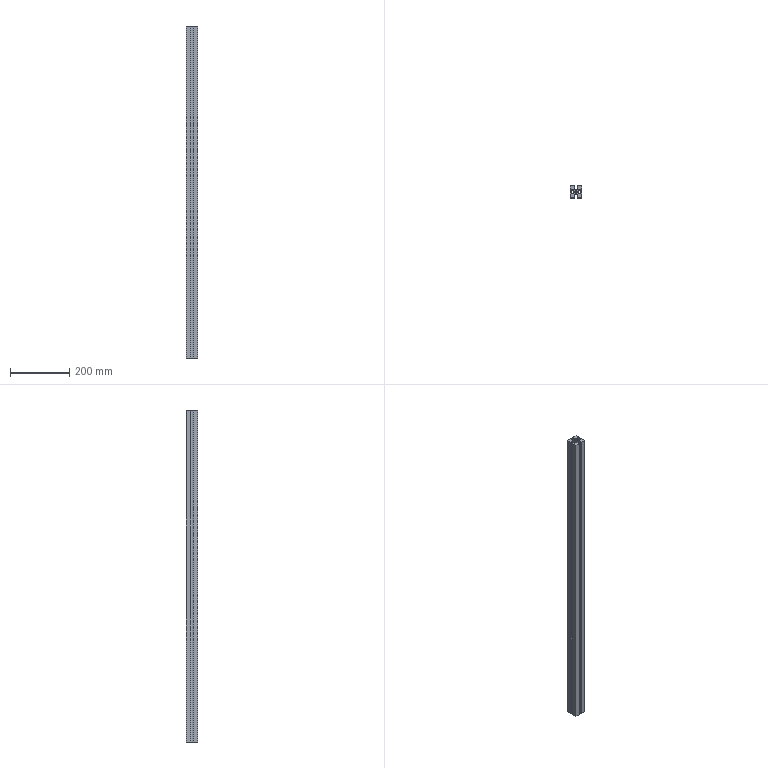Part | NX | 1 solid | 39 faces | box 40 x 40 x 1120 mm | volume 1079778 mm3 | plane 34 | cylinder 5 | commonest cylinder face diameters 19.333 x2 19.4 x2 6.8 x1
STEP:
#1=CARTESIAN_POINT('',(-125.,640.,-1120.));
#2=VERTEX_POINT('',#1);
#3=CARTESIAN_POINT('',(-125.,655.75,-1120.));
#4=VERTEX_POINT('',#3);
#5=CARTESIAN_POINT('',(-125.,640.5,-1120.));
#6=DIRECTION('',(0.,1.,0.));
#7=VECTOR('',#6,1000.);
#8=LINE('',#5,#7);
#9=EDGE_CURVE('',#2,#4,#8,.T.);
#10=ORIENTED_EDGE('',*,*,#9,.T.);
#11=CARTESIAN_POINT('',(-121.5,655.75,-1120.));
#12=VERTEX_POINT('',#11);
#13=CARTESIAN_POINT('',(-125.,655.75,-1120.));
#14=DIRECTION('',(1.,0.,0.));
#15=VECTOR('',#14,1000.);
#16=LINE('',#13,#15);
#17=EDGE_CURVE('',#4,#12,#16,.T.);
#18=ORIENTED_EDGE('',*,*,#17,.T.);
#19=CARTESIAN_POINT('',(-121.5,653.,-1120.));
#20=VERTEX_POINT('',#19);
#21=CARTESIAN_POINT('',(-121.5,655.75,-1120.));
#22=DIRECTION('',(0.,-1.,0.));
#23=VECTOR('',#22,1000.);
#24=LINE('',#21,#23);
#25=EDGE_CURVE('',#12,#20,#24,.T.);
#26=ORIENTED_EDGE('',*,*,#25,.T.);
#27=CARTESIAN_POINT('',(-114.5,653.,-1120.));
#28=VERTEX_POINT('',#27);
#29=CARTESIAN_POINT('',(-121.5,653.,-1120.));
#30=DIRECTION('',(1.,0.,0.));
#31=VECTOR('',#30,1000.);
#32=LINE('',#29,#31);
#33=EDGE_CURVE('',#20,#28,#32,.T.);
#34=ORIENTED_EDGE('',*,*,#33,.T.);
#35=CARTESIAN_POINT('',(-114.5,667.,-1120.));
#36=VERTEX_POINT('',#35);
#37=CARTESIAN_POINT('',(-121.167,660.,-1120.));
#38=DIRECTION('',(0.,0.,1.));
#39=DIRECTION('',(-1.,0.,0.));
#40=AXIS2_PLACEMENT_3D('',#37,#38,#39);
#41=CIRCLE('',#40,9.667);
#42=EDGE_CURVE('',#28,#36,#41,.T.);
#43=ORIENTED_EDGE('',*,*,#42,.T.);
#44=CARTESIAN_POINT('',(-121.5,667.,-1120.));
#45=VERTEX_POINT('',#44);
#46=CARTESIAN_POINT('',(-114.5,667.,-1120.));
#47=DIRECTION('',(-1.,0.,0.));
#48=VECTOR('',#47,1000.);
#49=LINE('',#46,#48);
#50=EDGE_CURVE('',#36,#45,#49,.T.);
#51=ORIENTED_EDGE('',*,*,#50,.T.);
#52=CARTESIAN_POINT('',(-121.5,664.25,-1120.));
#53=VERTEX_POINT('',#52);
#54=CARTESIAN_POINT('',(-121.5,667.,-1120.));
#55=DIRECTION('',(0.,-1.,0.));
#56=VECTOR('',#55,1000.);
#57=LINE('',#54,#56);
#58=EDGE_CURVE('',#45,#53,#57,.T.);
#59=ORIENTED_EDGE('',*,*,#58,.T.);
#60=CARTESIAN_POINT('',(-125.,664.25,-1120.));
#61=VERTEX_POINT('',#60);
#62=CARTESIAN_POINT('',(-121.5,664.25,-1120.));
#63=DIRECTION('',(-1.,0.,0.));
#64=VECTOR('',#63,1000.);
#65=LINE('',#62,#64);
#66=EDGE_CURVE('',#53,#61,#65,.T.);
#67=ORIENTED_EDGE('',*,*,#66,.T.);
#68=CARTESIAN_POINT('',(-125.,680.,-1120.));
#69=VERTEX_POINT('',#68);
#70=CARTESIAN_POINT('',(-125.,664.25,-1120.));
#71=DIRECTION('',(0.,1.,0.));
#72=VECTOR('',#71,1000.);
#73=LINE('',#70,#72);
#74=EDGE_CURVE('',#61,#69,#73,.T.);
#75=ORIENTED_EDGE('',*,*,#74,.T.);
#76=CARTESIAN_POINT('',(-109.25,680.,-1120.));
#77=VERTEX_POINT('',#76);
#78=CARTESIAN_POINT('',(-124.5,680.,-1120.));
#79=DIRECTION('',(1.,0.,0.));
#80=VECTOR('',#79,1000.);
#81=LINE('',#78,#80);
#82=EDGE_CURVE('',#69,#77,#81,.T.);
#83=ORIENTED_EDGE('',*,*,#82,.T.);
#84=CARTESIAN_POINT('',(-109.25,676.5,-1120.));
#85=VERTEX_POINT('',#84);
#86=CARTESIAN_POINT('',(-109.25,680.,-1120.));
#87=DIRECTION('',(0.,-1.,0.));
#88=VECTOR('',#87,1000.);
#89=LINE('',#86,#88);
#90=EDGE_CURVE('',#77,#85,#89,.T.);
#91=ORIENTED_EDGE('',*,*,#90,.T.);
#92=CARTESIAN_POINT('',(-111.5,676.5,-1120.));
#93=VERTEX_POINT('',#92);
#94=CARTESIAN_POINT('',(-109.25,676.5,-1120.));
#95=DIRECTION('',(-1.,0.,0.));
#96=VECTOR('',#95,1000.);
#97=LINE('',#94,#96);
#98=EDGE_CURVE('',#85,#93,#97,.T.);
#99=ORIENTED_EDGE('',*,*,#98,.T.);
#100=CARTESIAN_POINT('',(-111.5,669.5,-1120.));
#101=VERTEX_POINT('',#100);
#102=CARTESIAN_POINT('',(-111.5,676.5,-1120.));
#103=DIRECTION('',(0.,-1.,0.));
#104=VECTOR('',#103,1000.);
#105=LINE('',#102,#104);
#106=EDGE_CURVE('',#93,#101,#105,.T.);
#107=ORIENTED_EDGE('',*,*,#106,.T.);
#108=CARTESIAN_POINT('',(-98.5,669.5,-1120.));
#109=VERTEX_POINT('',#108);
#110=CARTESIAN_POINT('',(-105.,676.7,-1120.));
#111=DIRECTION('',(0.,0.,1.));
#112=DIRECTION('',(-1.,0.,0.));
#113=AXIS2_PLACEMENT_3D('',#110,#111,#112);
#114=CIRCLE('',#113,9.7);
#115=EDGE_CURVE('',#101,#109,#114,.T.);
#116=ORIENTED_EDGE('',*,*,#115,.T.);
#117=CARTESIAN_POINT('',(-98.5,676.5,-1120.));
#118=VERTEX_POINT('',#117);
#119=CARTESIAN_POINT('',(-98.5,669.5,-1120.));
#120=DIRECTION('',(0.,1.,0.));
#121=VECTOR('',#120,1000.);
#122=LINE('',#119,#121);
#123=EDGE_CURVE('',#109,#118,#122,.T.);
#124=ORIENTED_EDGE('',*,*,#123,.T.);
#125=CARTESIAN_POINT('',(-100.75,676.5,-1120.));
#126=VERTEX_POINT('',#125);
#127=CARTESIAN_POINT('',(-98.5,676.5,-1120.));
#128=DIRECTION('',(-1.,0.,0.));
#129=VECTOR('',#128,1000.);
#130=LINE('',#127,#129);
#131=EDGE_CURVE('',#118,#126,#130,.T.);
#132=ORIENTED_EDGE('',*,*,#131,.T.);
#133=CARTESIAN_POINT('',(-100.75,680.,-1120.));
#134=VERTEX_POINT('',#133);
#135=CARTESIAN_POINT('',(-100.75,676.5,-1120.));
#136=DIRECTION('',(0.,1.,0.));
#137=VECTOR('',#136,1000.);
#138=LINE('',#135,#137);
#139=EDGE_CURVE('',#126,#134,#138,.T.);
#140=ORIENTED_EDGE('',*,*,#139,.T.);
#141=CARTESIAN_POINT('',(-85.,680.,-1120.));
#142=VERTEX_POINT('',#141);
#143=CARTESIAN_POINT('',(-100.75,680.,-1120.));
#144=DIRECTION('',(1.,0.,0.));
#145=VECTOR('',#144,1000.);
#146=LINE('',#143,#145);
#147=EDGE_CURVE('',#134,#142,#146,.T.);
#148=ORIENTED_EDGE('',*,*,#147,.T.);
#149=CARTESIAN_POINT('',(-85.,664.25,-1120.));
#150=VERTEX_POINT('',#149);
#151=CARTESIAN_POINT('',(-85.,680.,-1120.));
#152=DIRECTION('',(0.,-1.,0.));
#153=VECTOR('',#152,1000.);
#154=LINE('',#151,#153);
#155=EDGE_CURVE('',#142,#150,#154,.T.);
#156=ORIENTED_EDGE('',*,*,#155,.T.);
#157=CARTESIAN_POINT('',(-88.5,664.25,-1120.));
#158=VERTEX_POINT('',#157);
#159=CARTESIAN_POINT('',(-85.,664.25,-1120.));
#160=DIRECTION('',(-1.,0.,0.));
#161=VECTOR('',#160,1000.);
#162=LINE('',#159,#161);
#163=EDGE_CURVE('',#150,#158,#162,.T.);
#164=ORIENTED_EDGE('',*,*,#163,.T.);
#165=CARTESIAN_POINT('',(-88.5,667.,-1120.));
#166=VERTEX_POINT('',#165);
#167=CARTESIAN_POINT('',(-88.5,664.25,-1120.));
#168=DIRECTION('',(0.,1.,0.));
#169=VECTOR('',#168,1000.);
#170=LINE('',#167,#169);
#171=EDGE_CURVE('',#158,#166,#170,.T.);
#172=ORIENTED_EDGE('',*,*,#171,.T.);
#173=CARTESIAN_POINT('',(-95.5,667.,-1120.));
#174=VERTEX_POINT('',#173);
#175=CARTESIAN_POINT('',(-88.5,667.,-1120.));
#176=DIRECTION('',(-1.,0.,0.));
#177=VECTOR('',#176,1000.);
#178=LINE('',#175,#177);
#179=EDGE_CURVE('',#166,#174,#178,.T.);
#180=ORIENTED_EDGE('',*,*,#179,.T.);
#181=CARTESIAN_POINT('',(-95.5,653.,-1120.));
#182=VERTEX_POINT('',#181);
#183=CARTESIAN_POINT('',(-88.833,660.,-1120.));
#184=DIRECTION('',(0.,0.,1.));
#185=DIRECTION('',(-1.,0.,0.));
#186=AXIS2_PLACEMENT_3D('',#183,#184,#185);
#187=CIRCLE('',#186,9.667);
#188=EDGE_CURVE('',#174,#182,#187,.T.);
#189=ORIENTED_EDGE('',*,*,#188,.T.);
#190=CARTESIAN_POINT('',(-88.5,653.,-1120.));
#191=VERTEX_POINT('',#190);
#192=CARTESIAN_POINT('',(-95.5,653.,-1120.));
#193=DIRECTION('',(1.,0.,0.));
#194=VECTOR('',#193,1000.);
#195=LINE('',#192,#194);
#196=EDGE_CURVE('',#182,#191,#195,.T.);
#197=ORIENTED_EDGE('',*,*,#196,.T.);
#198=CARTESIAN_POINT('',(-88.5,655.75,-1120.));
#199=VERTEX_POINT('',#198);
#200=CARTESIAN_POINT('',(-88.5,653.,-1120.));
#201=DIRECTION('',(0.,1.,0.));
#202=VECTOR('',#201,1000.);
#203=LINE('',#200,#202);
#204=EDGE_CURVE('',#191,#199,#203,.T.);
#205=ORIENTED_EDGE('',*,*,#204,.T.);
#206=CARTESIAN_POINT('',(-85.,655.75,-1120.));
#207=VERTEX_POINT('',#206);
#208=CARTESIAN_POINT('',(-88.5,655.75,-1120.));
#209=DIRECTION('',(1.,0.,0.));
#210=VECTOR('',#209,1000.);
#211=LINE('',#208,#210);
#212=EDGE_CURVE('',#199,#207,#211,.T.);
#213=ORIENTED_EDGE('',*,*,#212,.T.);
#214=CARTESIAN_POINT('',(-85.,640.,-1120.));
#215=VERTEX_POINT('',#214);
#216=CARTESIAN_POINT('',(-85.,655.75,-1120.));
#217=DIRECTION('',(0.,-1.,0.));
#218=VECTOR('',#217,1000.);
#219=LINE('',#216,#218);
#220=EDGE_CURVE('',#207,#215,#219,.T.);
#221=ORIENTED_EDGE('',*,*,#220,.T.);
#222=CARTESIAN_POINT('',(-100.75,640.,-1120.));
#223=VERTEX_POINT('',#222);
#224=CARTESIAN_POINT('',(-85.,640.,-1120.));
#225=DIRECTION('',(-1.,0.,0.));
#226=VECTOR('',#225,1000.);
#227=LINE('',#224,#226);
#228=EDGE_CURVE('',#215,#223,#227,.T.);
#229=ORIENTED_EDGE('',*,*,#228,.T.);
#230=CARTESIAN_POINT('',(-100.75,643.5,-1120.));
#231=VERTEX_POINT('',#230);
#232=CARTESIAN_POINT('',(-100.75,640.,-1120.));
#233=DIRECTION('',(0.,1.,0.));
#234=VECTOR('',#233,1000.);
#235=LINE('',#232,#234);
#236=EDGE_CURVE('',#223,#231,#235,.T.);
#237=ORIENTED_EDGE('',*,*,#236,.T.);
#238=CARTESIAN_POINT('',(-98.5,643.5,-1120.));
#239=VERTEX_POINT('',#238);
#240=CARTESIAN_POINT('',(-100.75,643.5,-1120.));
#241=DIRECTION('',(1.,0.,0.));
#242=VECTOR('',#241,1000.);
#243=LINE('',#240,#242);
#244=EDGE_CURVE('',#231,#239,#243,.T.);
#245=ORIENTED_EDGE('',*,*,#244,.T.);
#246=CARTESIAN_POINT('',(-98.5,650.5,-1120.));
#247=VERTEX_POINT('',#246);
#248=CARTESIAN_POINT('',(-98.5,643.5,-1120.));
#249=DIRECTION('',(0.,1.,0.));
#250=VECTOR('',#249,1000.);
#251=LINE('',#248,#250);
#252=EDGE_CURVE('',#239,#247,#251,.T.);
#253=ORIENTED_EDGE('',*,*,#252,.T.);
#254=CARTESIAN_POINT('',(-111.5,650.5,-1120.));
#255=VERTEX_POINT('',#254);
#256=CARTESIAN_POINT('',(-105.,643.3,-1120.));
#257=DIRECTION('',(0.,0.,1.));
#258=DIRECTION('',(-1.,0.,0.));
#259=AXIS2_PLACEMENT_3D('',#256,#257,#258);
#260=CIRCLE('',#259,9.7);
#261=EDGE_CURVE('',#247,#255,#260,.T.);
#262=ORIENTED_EDGE('',*,*,#261,.T.);
#263=CARTESIAN_POINT('',(-111.5,643.5,-1120.));
#264=VERTEX_POINT('',#263);
#265=CARTESIAN_POINT('',(-111.5,650.5,-1120.));
#266=DIRECTION('',(0.,-1.,0.));
#267=VECTOR('',#266,1000.);
#268=LINE('',#265,#267);
#269=EDGE_CURVE('',#255,#264,#268,.T.);
#270=ORIENTED_EDGE('',*,*,#269,.T.);
#271=CARTESIAN_POINT('',(-109.25,643.5,-1120.));
#272=VERTEX_POINT('',#271);
#273=CARTESIAN_POINT('',(-111.5,643.5,-1120.));
#274=DIRECTION('',(1.,0.,0.));
#275=VECTOR('',#274,1000.);
#276=LINE('',#273,#275);
#277=EDGE_CURVE('',#264,#272,#276,.T.);
#278=ORIENTED_EDGE('',*,*,#277,.T.);
#279=CARTESIAN_POINT('',(-109.25,640.,-1120.));
#280=VERTEX_POINT('',#279);
#281=CARTESIAN_POINT('',(-109.25,643.5,-1120.));
#282=DIRECTION('',(0.,-1.,0.));
#283=VECTOR('',#282,1000.);
#284=LINE('',#281,#283);
#285=EDGE_CURVE('',#272,#280,#284,.T.);
#286=ORIENTED_EDGE('',*,*,#285,.T.);
#287=CARTESIAN_POINT('',(-109.25,640.,-1120.));
#288=DIRECTION('',(-1.,0.,0.));
#289=VECTOR('',#288,1000.);
#290=LINE('',#287,#289);
#291=EDGE_CURVE('',#280,#2,#290,.T.);
#292=ORIENTED_EDGE('',*,*,#291,.T.);
#293=EDGE_LOOP('',(#10,#18,#26,#34,#43,#51,#59,#67,#75,#83,#91,#99,#107,#116,#124,#132,#140,#148,#156,#164,#172,#180,#189,#197,#205,#213,#221,#229,#237,#245,#253,#262,#270,#278,#286,#292));
#294=FACE_BOUND('',#293,.T.);
#295=CARTESIAN_POINT('',(-108.4,660.,-1120.));
#296=VERTEX_POINT('',#295);
#297=CARTESIAN_POINT('',(-105.,660.,-1120.));
#298=DIRECTION('',(0.,0.,-1.));
#299=DIRECTION('',(-1.,0.,0.));
#300=AXIS2_PLACEMENT_3D('',#297,#298,#299);
#301=CIRCLE('',#300,3.4);
#302=EDGE_CURVE('',#296,#296,#301,.T.);
#303=ORIENTED_EDGE('',*,*,#302,.F.);
#304=EDGE_LOOP('',(#303));
#305=FACE_BOUND('',#304,.T.);
#306=CARTESIAN_POINT('',(-121.167,660.,-1120.));
#307=DIRECTION('',(0.,0.,-1.));
#308=DIRECTION('',(-1.,0.,0.));
#309=AXIS2_PLACEMENT_3D('',#306,#307,#308);
#310=PLANE('',#309);
#311=ADVANCED_FACE('',(#294,#305),#310,.T.);
#312=CARTESIAN_POINT('',(-125.,655.75,0.));
#313=VERTEX_POINT('',#312);
#314=CARTESIAN_POINT('',(-121.5,655.75,0.));
#315=VERTEX_POINT('',#314);
#316=CARTESIAN_POINT('',(-125.,655.75,0.));
#317=DIRECTION('',(1.,0.,0.));
#318=VECTOR('',#317,1000.);
#319=LINE('',#316,#318);
#320=EDGE_CURVE('',#313,#315,#319,.T.);
#321=ORIENTED_EDGE('',*,*,#320,.F.);
#322=CARTESIAN_POINT('',(-125.,640.,0.));
#323=VERTEX_POINT('',#322);
#324=CARTESIAN_POINT('',(-125.,640.5,0.));
#325=DIRECTION('',(0.,1.,0.));
#326=VECTOR('',#325,1000.);
#327=LINE('',#324,#326);
#328=EDGE_CURVE('',#323,#313,#327,.T.);
#329=ORIENTED_EDGE('',*,*,#328,.F.);
#330=CARTESIAN_POINT('',(-109.25,640.,0.));
#331=VERTEX_POINT('',#330);
#332=CARTESIAN_POINT('',(-125.,640.,0.));
#333=DIRECTION('',(-1.,0.,0.));
#334=VECTOR('',#333,1000.);
#335=LINE('',#332,#334);
#336=EDGE_CURVE('',#331,#323,#335,.T.);
#337=ORIENTED_EDGE('',*,*,#336,.F.);
#338=CARTESIAN_POINT('',(-109.25,643.5,0.));
#339=VERTEX_POINT('',#338);
#340=CARTESIAN_POINT('',(-109.25,643.5,0.));
#341=DIRECTION('',(0.,-1.,0.));
#342=VECTOR('',#341,1000.);
#343=LINE('',#340,#342);
#344=EDGE_CURVE('',#339,#331,#343,.T.);
#345=ORIENTED_EDGE('',*,*,#344,.F.);
#346=CARTESIAN_POINT('',(-111.5,643.5,0.));
#347=VERTEX_POINT('',#346);
#348=CARTESIAN_POINT('',(-111.5,643.5,0.));
#349=DIRECTION('',(1.,0.,0.));
#350=VECTOR('',#349,1000.);
#351=LINE('',#348,#350);
#352=EDGE_CURVE('',#347,#339,#351,.T.);
#353=ORIENTED_EDGE('',*,*,#352,.F.);
#354=CARTESIAN_POINT('',(-111.5,650.5,0.));
#355=VERTEX_POINT('',#354);
#356=CARTESIAN_POINT('',(-111.5,650.5,0.));
#357=DIRECTION('',(0.,-1.,0.));
#358=VECTOR('',#357,1000.);
#359=LINE('',#356,#358);
#360=EDGE_CURVE('',#355,#347,#359,.T.);
#361=ORIENTED_EDGE('',*,*,#360,.F.);
#362=CARTESIAN_POINT('',(-98.5,650.5,0.));
#363=VERTEX_POINT('',#362);
#364=CARTESIAN_POINT('',(-105.,643.3,0.));
#365=DIRECTION('',(0.,0.,1.));
#366=DIRECTION('',(-1.,0.,0.));
#367=AXIS2_PLACEMENT_3D('',#364,#365,#366);
#368=CIRCLE('',#367,9.7);
#369=EDGE_CURVE('',#363,#355,#368,.T.);
#370=ORIENTED_EDGE('',*,*,#369,.F.);
#371=CARTESIAN_POINT('',(-98.5,643.5,0.));
#372=VERTEX_POINT('',#371);
#373=CARTESIAN_POINT('',(-98.5,643.5,0.));
#374=DIRECTION('',(0.,1.,0.));
#375=VECTOR('',#374,1000.);
#376=LINE('',#373,#375);
#377=EDGE_CURVE('',#372,#363,#376,.T.);
#378=ORIENTED_EDGE('',*,*,#377,.F.);
#379=CARTESIAN_POINT('',(-100.75,643.5,0.));
#380=VERTEX_POINT('',#379);
#381=CARTESIAN_POINT('',(-100.75,643.5,0.));
#382=DIRECTION('',(1.,0.,0.));
#383=VECTOR('',#382,1000.);
#384=LINE('',#381,#383);
#385=EDGE_CURVE('',#380,#372,#384,.T.);
#386=ORIENTED_EDGE('',*,*,#385,.F.);
#387=CARTESIAN_POINT('',(-100.75,640.,0.));
#388=VERTEX_POINT('',#387);
#389=CARTESIAN_POINT('',(-100.75,640.,0.));
#390=DIRECTION('',(0.,1.,0.));
#391=VECTOR('',#390,1000.);
#392=LINE('',#389,#391);
#393=EDGE_CURVE('',#388,#380,#392,.T.);
#394=ORIENTED_EDGE('',*,*,#393,.F.);
#395=CARTESIAN_POINT('',(-85.,640.,0.));
#396=VERTEX_POINT('',#395);
#397=CARTESIAN_POINT('',(-85.5,640.,0.));
#398=DIRECTION('',(-1.,0.,0.));
#399=VECTOR('',#398,1000.);
#400=LINE('',#397,#399);
#401=EDGE_CURVE('',#396,#388,#400,.T.);
#402=ORIENTED_EDGE('',*,*,#401,.F.);
#403=CARTESIAN_POINT('',(-85.,655.75,0.));
#404=VERTEX_POINT('',#403);
#405=CARTESIAN_POINT('',(-85.,640.5,0.));
#406=DIRECTION('',(0.,-1.,0.));
#407=VECTOR('',#406,1000.);
#408=LINE('',#405,#407);
#409=EDGE_CURVE('',#404,#396,#408,.T.);
#410=ORIENTED_EDGE('',*,*,#409,.F.);
#411=CARTESIAN_POINT('',(-88.5,655.75,0.));
#412=VERTEX_POINT('',#411);
#413=CARTESIAN_POINT('',(-88.5,655.75,0.));
#414=DIRECTION('',(1.,0.,0.));
#415=VECTOR('',#414,1000.);
#416=LINE('',#413,#415);
#417=EDGE_CURVE('',#412,#404,#416,.T.);
#418=ORIENTED_EDGE('',*,*,#417,.F.);
#419=CARTESIAN_POINT('',(-88.5,653.,0.));
#420=VERTEX_POINT('',#419);
#421=CARTESIAN_POINT('',(-88.5,653.,0.));
#422=DIRECTION('',(0.,1.,0.));
#423=VECTOR('',#422,1000.);
#424=LINE('',#421,#423);
#425=EDGE_CURVE('',#420,#412,#424,.T.);
#426=ORIENTED_EDGE('',*,*,#425,.F.);
#427=CARTESIAN_POINT('',(-95.5,653.,0.));
#428=VERTEX_POINT('',#427);
#429=CARTESIAN_POINT('',(-95.5,653.,0.));
#430=DIRECTION('',(1.,0.,0.));
#431=VECTOR('',#430,1000.);
#432=LINE('',#429,#431);
#433=EDGE_CURVE('',#428,#420,#432,.T.);
#434=ORIENTED_EDGE('',*,*,#433,.F.);
#435=CARTESIAN_POINT('',(-95.5,667.,0.));
#436=VERTEX_POINT('',#435);
#437=CARTESIAN_POINT('',(-88.833,660.,0.));
#438=DIRECTION('',(0.,0.,1.));
#439=DIRECTION('',(-1.,0.,0.));
#440=AXIS2_PLACEMENT_3D('',#437,#438,#439);
#441=CIRCLE('',#440,9.667);
#442=EDGE_CURVE('',#436,#428,#441,.T.);
#443=ORIENTED_EDGE('',*,*,#442,.F.);
#444=CARTESIAN_POINT('',(-88.5,667.,0.));
#445=VERTEX_POINT('',#444);
#446=CARTESIAN_POINT('',(-88.5,667.,0.));
#447=DIRECTION('',(-1.,0.,0.));
#448=VECTOR('',#447,1000.);
#449=LINE('',#446,#448);
#450=EDGE_CURVE('',#445,#436,#449,.T.);
#451=ORIENTED_EDGE('',*,*,#450,.F.);
#452=CARTESIAN_POINT('',(-88.5,664.25,0.));
#453=VERTEX_POINT('',#452);
#454=CARTESIAN_POINT('',(-88.5,664.25,0.));
#455=DIRECTION('',(0.,1.,0.));
#456=VECTOR('',#455,1000.);
#457=LINE('',#454,#456);
#458=EDGE_CURVE('',#453,#445,#457,.T.);
#459=ORIENTED_EDGE('',*,*,#458,.F.);
#460=CARTESIAN_POINT('',(-85.,664.25,0.));
#461=VERTEX_POINT('',#460);
#462=CARTESIAN_POINT('',(-85.,664.25,0.));
#463=DIRECTION('',(-1.,0.,0.));
#464=VECTOR('',#463,1000.);
#465=LINE('',#462,#464);
#466=EDGE_CURVE('',#461,#453,#465,.T.);
#467=ORIENTED_EDGE('',*,*,#466,.F.);
#468=CARTESIAN_POINT('',(-85.,680.,0.));
#469=VERTEX_POINT('',#468);
#470=CARTESIAN_POINT('',(-85.,679.5,0.));
#471=DIRECTION('',(0.,-1.,0.));
#472=VECTOR('',#471,1000.);
#473=LINE('',#470,#472);
#474=EDGE_CURVE('',#469,#461,#473,.T.);
#475=ORIENTED_EDGE('',*,*,#474,.F.);
#476=CARTESIAN_POINT('',(-100.75,680.,0.));
#477=VERTEX_POINT('',#476);
#478=CARTESIAN_POINT('',(-85.5,680.,0.));
#479=DIRECTION('',(1.,0.,0.));
#480=VECTOR('',#479,1000.);
#481=LINE('',#478,#480);
#482=EDGE_CURVE('',#477,#469,#481,.T.);
#483=ORIENTED_EDGE('',*,*,#482,.F.);
#484=CARTESIAN_POINT('',(-100.75,676.5,0.));
#485=VERTEX_POINT('',#484);
#486=CARTESIAN_POINT('',(-100.75,676.5,0.));
#487=DIRECTION('',(0.,1.,0.));
#488=VECTOR('',#487,1000.);
#489=LINE('',#486,#488);
#490=EDGE_CURVE('',#485,#477,#489,.T.);
#491=ORIENTED_EDGE('',*,*,#490,.F.);
#492=CARTESIAN_POINT('',(-98.5,676.5,0.));
#493=VERTEX_POINT('',#492);
#494=CARTESIAN_POINT('',(-98.5,676.5,0.));
#495=DIRECTION('',(-1.,0.,0.));
#496=VECTOR('',#495,1000.);
#497=LINE('',#494,#496);
#498=EDGE_CURVE('',#493,#485,#497,.T.);
#499=ORIENTED_EDGE('',*,*,#498,.F.);
#500=CARTESIAN_POINT('',(-98.5,669.5,0.));
#501=VERTEX_POINT('',#500);
#502=CARTESIAN_POINT('',(-98.5,669.5,0.));
#503=DIRECTION('',(0.,1.,0.));
#504=VECTOR('',#503,1000.);
#505=LINE('',#502,#504);
#506=EDGE_CURVE('',#501,#493,#505,.T.);
#507=ORIENTED_EDGE('',*,*,#506,.F.);
#508=CARTESIAN_POINT('',(-111.5,669.5,0.));
#509=VERTEX_POINT('',#508);
#510=CARTESIAN_POINT('',(-105.,676.7,0.));
#511=DIRECTION('',(0.,0.,1.));
#512=DIRECTION('',(-1.,0.,0.));
#513=AXIS2_PLACEMENT_3D('',#510,#511,#512);
#514=CIRCLE('',#513,9.7);
#515=EDGE_CURVE('',#509,#501,#514,.T.);
#516=ORIENTED_EDGE('',*,*,#515,.F.);
#517=CARTESIAN_POINT('',(-111.5,676.5,0.));
#518=VERTEX_POINT('',#517);
#519=CARTESIAN_POINT('',(-111.5,676.5,0.));
#520=DIRECTION('',(0.,-1.,0.));
#521=VECTOR('',#520,1000.);
#522=LINE('',#519,#521);
#523=EDGE_CURVE('',#518,#509,#522,.T.);
#524=ORIENTED_EDGE('',*,*,#523,.F.);
#525=CARTESIAN_POINT('',(-109.25,676.5,0.));
#526=VERTEX_POINT('',#525);
#527=CARTESIAN_POINT('',(-109.25,676.5,0.));
#528=DIRECTION('',(-1.,0.,0.));
#529=VECTOR('',#528,1000.);
#530=LINE('',#527,#529);
#531=EDGE_CURVE('',#526,#518,#530,.T.);
#532=ORIENTED_EDGE('',*,*,#531,.F.);
#533=CARTESIAN_POINT('',(-109.25,680.,0.));
#534=VERTEX_POINT('',#533);
#535=CARTESIAN_POINT('',(-109.25,680.,0.));
#536=DIRECTION('',(0.,-1.,0.));
#537=VECTOR('',#536,1000.);
#538=LINE('',#535,#537);
#539=EDGE_CURVE('',#534,#526,#538,.T.);
#540=ORIENTED_EDGE('',*,*,#539,.F.);
#541=CARTESIAN_POINT('',(-125.,680.,0.));
#542=VERTEX_POINT('',#541);
#543=CARTESIAN_POINT('',(-124.5,680.,0.));
#544=DIRECTION('',(1.,0.,0.));
#545=VECTOR('',#544,1000.);
#546=LINE('',#543,#545);
#547=EDGE_CURVE('',#542,#534,#546,.T.);
#548=ORIENTED_EDGE('',*,*,#547,.F.);
#549=CARTESIAN_POINT('',(-125.,664.25,0.));
#550=VERTEX_POINT('',#549);
#551=CARTESIAN_POINT('',(-125.,680.,0.));
#552=DIRECTION('',(0.,1.,0.));
#553=VECTOR('',#552,1000.);
#554=LINE('',#551,#553);
#555=EDGE_CURVE('',#550,#542,#554,.T.);
#556=ORIENTED_EDGE('',*,*,#555,.F.);
#557=CARTESIAN_POINT('',(-121.5,664.25,0.));
#558=VERTEX_POINT('',#557);
#559=CARTESIAN_POINT('',(-121.5,664.25,0.));
#560=DIRECTION('',(-1.,0.,0.));
#561=VECTOR('',#560,1000.);
#562=LINE('',#559,#561);
#563=EDGE_CURVE('',#558,#550,#562,.T.);
#564=ORIENTED_EDGE('',*,*,#563,.F.);
#565=CARTESIAN_POINT('',(-121.5,667.,0.));
#566=VERTEX_POINT('',#565);
#567=CARTESIAN_POINT('',(-121.5,667.,0.));
#568=DIRECTION('',(0.,-1.,0.));
#569=VECTOR('',#568,1000.);
#570=LINE('',#567,#569);
#571=EDGE_CURVE('',#566,#558,#570,.T.);
#572=ORIENTED_EDGE('',*,*,#571,.F.);
#573=CARTESIAN_POINT('',(-114.5,667.,0.));
#574=VERTEX_POINT('',#573);
#575=CARTESIAN_POINT('',(-114.5,667.,0.));
#576=DIRECTION('',(-1.,0.,0.));
#577=VECTOR('',#576,1000.);
#578=LINE('',#575,#577);
#579=EDGE_CURVE('',#574,#566,#578,.T.);
#580=ORIENTED_EDGE('',*,*,#579,.F.);
#581=CARTESIAN_POINT('',(-114.5,653.,0.));
#582=VERTEX_POINT('',#581);
#583=CARTESIAN_POINT('',(-121.167,660.,0.));
#584=DIRECTION('',(0.,0.,1.));
#585=DIRECTION('',(-1.,0.,0.));
#586=AXIS2_PLACEMENT_3D('',#583,#584,#585);
#587=CIRCLE('',#586,9.667);
#588=EDGE_CURVE('',#582,#574,#587,.T.);
#589=ORIENTED_EDGE('',*,*,#588,.F.);
#590=CARTESIAN_POINT('',(-121.5,653.,0.));
#591=VERTEX_POINT('',#590);
#592=CARTESIAN_POINT('',(-121.5,653.,0.));
#593=DIRECTION('',(1.,0.,0.));
#594=VECTOR('',#593,1000.);
#595=LINE('',#592,#594);
#596=EDGE_CURVE('',#591,#582,#595,.T.);
#597=ORIENTED_EDGE('',*,*,#596,.F.);
#598=CARTESIAN_POINT('',(-121.5,655.75,0.));
#599=DIRECTION('',(0.,-1.,0.));
#600=VECTOR('',#599,1000.);
#601=LINE('',#598,#600);
#602=EDGE_CURVE('',#315,#591,#601,.T.);
#603=ORIENTED_EDGE('',*,*,#602,.F.);
#604=EDGE_LOOP('',(#321,#329,#337,#345,#353,#361,#370,#378,#386,#394,#402,#410,#418,#426,#434,#443,#451,#459,#467,#475,#483,#491,#499,#507,#516,#524,#532,#540,#548,#556,#564,#572,#580,#589,#597,#603));
#605=FACE_BOUND('',#604,.T.);
#606=CARTESIAN_POINT('',(-108.4,660.,0.));
#607=VERTEX_POINT('',#606);
#608=CARTESIAN_POINT('',(-105.,660.,0.));
#609=DIRECTION('',(0.,0.,-1.));
#610=DIRECTION('',(-1.,0.,0.));
#611=AXIS2_PLACEMENT_3D('',#608,#609,#610);
#612=CIRCLE('',#611,3.4);
#613=EDGE_CURVE('',#607,#607,#612,.T.);
#614=ORIENTED_EDGE('',*,*,#613,.T.);
#615=EDGE_LOOP('',(#614));
#616=FACE_BOUND('',#615,.T.);
#617=CARTESIAN_POINT('',(-121.167,660.,0.));
#618=DIRECTION('',(0.,0.,-1.));
#619=DIRECTION('',(-1.,0.,0.));
#620=AXIS2_PLACEMENT_3D('',#617,#618,#619);
#621=PLANE('',#620);
#622=ADVANCED_FACE('',(#605,#616),#621,.F.);
#623=ORIENTED_EDGE('',*,*,#320,.T.);
#624=CARTESIAN_POINT('',(-121.5,655.75,-1120.));
#625=DIRECTION('',(0.,0.,1.));
#626=VECTOR('',#625,1000.);
#627=LINE('',#624,#626);
#628=EDGE_CURVE('',#12,#315,#627,.T.);
#629=ORIENTED_EDGE('',*,*,#628,.F.);
#630=ORIENTED_EDGE('',*,*,#17,.F.);
#631=CARTESIAN_POINT('',(-125.,655.75,-1120.));
#632=DIRECTION('',(0.,0.,1.));
#633=VECTOR('',#632,1000.);
#634=LINE('',#631,#633);
#635=EDGE_CURVE('',#4,#313,#634,.T.);
#636=ORIENTED_EDGE('',*,*,#635,.T.);
#637=EDGE_LOOP('',(#623,#629,#630,#636));
#638=FACE_BOUND('',#637,.T.);
#639=CARTESIAN_POINT('',(-125.,655.75,-1120.));
#640=DIRECTION('',(0.,-1.,0.));
#641=DIRECTION('',(0.,0.,-1.));
#642=AXIS2_PLACEMENT_3D('',#639,#640,#641);
#643=PLANE('',#642);
#644=ADVANCED_FACE('',(#638),#643,.F.);
#645=ORIENTED_EDGE('',*,*,#602,.T.);
#646=CARTESIAN_POINT('',(-121.5,653.,-1120.));
#647=DIRECTION('',(0.,0.,1.));
#648=VECTOR('',#647,1000.);
#649=LINE('',#646,#648);
#650=EDGE_CURVE('',#20,#591,#649,.T.);
#651=ORIENTED_EDGE('',*,*,#650,.F.);
#652=ORIENTED_EDGE('',*,*,#25,.F.);
#653=ORIENTED_EDGE('',*,*,#628,.T.);
#654=EDGE_LOOP('',(#645,#651,#652,#653));
#655=FACE_BOUND('',#654,.T.);
#656=CARTESIAN_POINT('',(-121.5,655.75,-1120.));
#657=DIRECTION('',(-1.,0.,0.));
#658=DIRECTION('',(0.,0.,1.));
#659=AXIS2_PLACEMENT_3D('',#656,#657,#658);
#660=PLANE('',#659);
#661=ADVANCED_FACE('',(#655),#660,.F.);
#662=ORIENTED_EDGE('',*,*,#596,.T.);
#663=CARTESIAN_POINT('',(-114.5,653.,-1120.));
#664=DIRECTION('',(0.,0.,1.));
#665=VECTOR('',#664,1000.);
#666=LINE('',#663,#665);
#667=EDGE_CURVE('',#28,#582,#666,.T.);
#668=ORIENTED_EDGE('',*,*,#667,.F.);
#669=ORIENTED_EDGE('',*,*,#33,.F.);
#670=ORIENTED_EDGE('',*,*,#650,.T.);
#671=EDGE_LOOP('',(#662,#668,#669,#670));
#672=FACE_BOUND('',#671,.T.);
#673=CARTESIAN_POINT('',(-121.5,653.,-1120.));
#674=DIRECTION('',(0.,-1.,0.));
#675=DIRECTION('',(0.,0.,-1.));
#676=AXIS2_PLACEMENT_3D('',#673,#674,#675);
#677=PLANE('',#676);
#678=ADVANCED_FACE('',(#672),#677,.F.);
#679=ORIENTED_EDGE('',*,*,#588,.T.);
#680=CARTESIAN_POINT('',(-114.5,667.,-1120.));
#681=DIRECTION('',(0.,0.,1.));
#682=VECTOR('',#681,1000.);
#683=LINE('',#680,#682);
#684=EDGE_CURVE('',#36,#574,#683,.T.);
#685=ORIENTED_EDGE('',*,*,#684,.F.);
#686=ORIENTED_EDGE('',*,*,#42,.F.);
#687=ORIENTED_EDGE('',*,*,#667,.T.);
#688=EDGE_LOOP('',(#679,#685,#686,#687));
#689=FACE_BOUND('',#688,.T.);
#690=CARTESIAN_POINT('',(-121.167,660.,-1120.));
#691=DIRECTION('',(0.,0.,1.));
#692=DIRECTION('',(1.,0.,0.));
#693=AXIS2_PLACEMENT_3D('',#690,#691,#692);
#694=CYLINDRICAL_SURFACE('',#693,9.667);
#695=ADVANCED_FACE('',(#689),#694,.F.);
#696=ORIENTED_EDGE('',*,*,#579,.T.);
#697=CARTESIAN_POINT('',(-121.5,667.,-1120.));
#698=DIRECTION('',(0.,0.,1.));
#699=VECTOR('',#698,1000.);
#700=LINE('',#697,#699);
#701=EDGE_CURVE('',#45,#566,#700,.T.);
#702=ORIENTED_EDGE('',*,*,#701,.F.);
#703=ORIENTED_EDGE('',*,*,#50,.F.);
#704=ORIENTED_EDGE('',*,*,#684,.T.);
#705=EDGE_LOOP('',(#696,#702,#703,#704));
#706=FACE_BOUND('',#705,.T.);
#707=CARTESIAN_POINT('',(-114.5,667.,-1120.));
#708=DIRECTION('',(0.,1.,0.));
#709=DIRECTION('',(0.,0.,1.));
#710=AXIS2_PLACEMENT_3D('',#707,#708,#709);
#711=PLANE('',#710);
#712=ADVANCED_FACE('',(#706),#711,.F.);
#713=ORIENTED_EDGE('',*,*,#571,.T.);
#714=CARTESIAN_POINT('',(-121.5,664.25,-1120.));
#715=DIRECTION('',(0.,0.,1.));
#716=VECTOR('',#715,1000.);
#717=LINE('',#714,#716);
#718=EDGE_CURVE('',#53,#558,#717,.T.);
#719=ORIENTED_EDGE('',*,*,#718,.F.);
#720=ORIENTED_EDGE('',*,*,#58,.F.);
#721=ORIENTED_EDGE('',*,*,#701,.T.);
#722=EDGE_LOOP('',(#713,#719,#720,#721));
#723=FACE_BOUND('',#722,.T.);
#724=CARTESIAN_POINT('',(-121.5,667.,-1120.));
#725=DIRECTION('',(-1.,0.,0.));
#726=DIRECTION('',(0.,0.,1.));
#727=AXIS2_PLACEMENT_3D('',#724,#725,#726);
#728=PLANE('',#727);
#729=ADVANCED_FACE('',(#723),#728,.F.);
#730=ORIENTED_EDGE('',*,*,#563,.T.);
#731=CARTESIAN_POINT('',(-125.,664.25,-1120.));
#732=DIRECTION('',(0.,0.,1.));
#733=VECTOR('',#732,1000.);
#734=LINE('',#731,#733);
#735=EDGE_CURVE('',#61,#550,#734,.T.);
#736=ORIENTED_EDGE('',*,*,#735,.F.);
#737=ORIENTED_EDGE('',*,*,#66,.F.);
#738=ORIENTED_EDGE('',*,*,#718,.T.);
#739=EDGE_LOOP('',(#730,#736,#737,#738));
#740=FACE_BOUND('',#739,.T.);
#741=CARTESIAN_POINT('',(-121.5,664.25,-1120.));
#742=DIRECTION('',(0.,1.,0.));
#743=DIRECTION('',(0.,0.,1.));
#744=AXIS2_PLACEMENT_3D('',#741,#742,#743);
#745=PLANE('',#744);
#746=ADVANCED_FACE('',(#740),#745,.F.);
#747=ORIENTED_EDGE('',*,*,#555,.T.);
#748=CARTESIAN_POINT('',(-125.,680.,-1120.));
#749=DIRECTION('',(0.,0.,1.));
#750=VECTOR('',#749,1000.);
#751=LINE('',#748,#750);
#752=EDGE_CURVE('',#69,#542,#751,.T.);
#753=ORIENTED_EDGE('',*,*,#752,.F.);
#754=ORIENTED_EDGE('',*,*,#74,.F.);
#755=ORIENTED_EDGE('',*,*,#735,.T.);
#756=EDGE_LOOP('',(#747,#753,#754,#755));
#757=FACE_BOUND('',#756,.T.);
#758=CARTESIAN_POINT('',(-125.,680.,-1120.));
#759=DIRECTION('',(1.,0.,0.));
#760=DIRECTION('',(0.,0.,-1.));
#761=AXIS2_PLACEMENT_3D('',#758,#759,#760);
#762=PLANE('',#761);
#763=ADVANCED_FACE('',(#757),#762,.F.);
#764=ORIENTED_EDGE('',*,*,#547,.T.);
#765=CARTESIAN_POINT('',(-109.25,680.,-1120.));
#766=DIRECTION('',(0.,0.,1.));
#767=VECTOR('',#766,1000.);
#768=LINE('',#765,#767);
#769=EDGE_CURVE('',#77,#534,#768,.T.);
#770=ORIENTED_EDGE('',*,*,#769,.F.);
#771=ORIENTED_EDGE('',*,*,#82,.F.);
#772=ORIENTED_EDGE('',*,*,#752,.T.);
#773=EDGE_LOOP('',(#764,#770,#771,#772));
#774=FACE_BOUND('',#773,.T.);
#775=CARTESIAN_POINT('',(-124.5,680.,-1120.));
#776=DIRECTION('',(0.,-1.,0.));
#777=DIRECTION('',(0.,0.,-1.));
#778=AXIS2_PLACEMENT_3D('',#775,#776,#777);
#779=PLANE('',#778);
#780=ADVANCED_FACE('',(#774),#779,.F.);
#781=ORIENTED_EDGE('',*,*,#539,.T.);
#782=CARTESIAN_POINT('',(-109.25,676.5,-1120.));
#783=DIRECTION('',(0.,0.,1.));
#784=VECTOR('',#783,1000.);
#785=LINE('',#782,#784);
#786=EDGE_CURVE('',#85,#526,#785,.T.);
#787=ORIENTED_EDGE('',*,*,#786,.F.);
#788=ORIENTED_EDGE('',*,*,#90,.F.);
#789=ORIENTED_EDGE('',*,*,#769,.T.);
#790=EDGE_LOOP('',(#781,#787,#788,#789));
#791=FACE_BOUND('',#790,.T.);
#792=CARTESIAN_POINT('',(-109.25,680.,-1120.));
#793=DIRECTION('',(-1.,0.,0.));
#794=DIRECTION('',(0.,0.,1.));
#795=AXIS2_PLACEMENT_3D('',#792,#793,#794);
#796=PLANE('',#795);
#797=ADVANCED_FACE('',(#791),#796,.F.);
#798=ORIENTED_EDGE('',*,*,#531,.T.);
#799=CARTESIAN_POINT('',(-111.5,676.5,-1120.));
#800=DIRECTION('',(0.,0.,1.));
#801=VECTOR('',#800,1000.);
#802=LINE('',#799,#801);
#803=EDGE_CURVE('',#93,#518,#802,.T.);
#804=ORIENTED_EDGE('',*,*,#803,.F.);
#805=ORIENTED_EDGE('',*,*,#98,.F.);
#806=ORIENTED_EDGE('',*,*,#786,.T.);
#807=EDGE_LOOP('',(#798,#804,#805,#806));
#808=FACE_BOUND('',#807,.T.);
#809=CARTESIAN_POINT('',(-109.25,676.5,-1120.));
#810=DIRECTION('',(0.,1.,0.));
#811=DIRECTION('',(0.,0.,1.));
#812=AXIS2_PLACEMENT_3D('',#809,#810,#811);
#813=PLANE('',#812);
#814=ADVANCED_FACE('',(#808),#813,.F.);
#815=ORIENTED_EDGE('',*,*,#523,.T.);
#816=CARTESIAN_POINT('',(-111.5,669.5,-1120.));
#817=DIRECTION('',(0.,0.,1.));
#818=VECTOR('',#817,1000.);
#819=LINE('',#816,#818);
#820=EDGE_CURVE('',#101,#509,#819,.T.);
#821=ORIENTED_EDGE('',*,*,#820,.F.);
#822=ORIENTED_EDGE('',*,*,#106,.F.);
#823=ORIENTED_EDGE('',*,*,#803,.T.);
#824=EDGE_LOOP('',(#815,#821,#822,#823));
#825=FACE_BOUND('',#824,.T.);
#826=CARTESIAN_POINT('',(-111.5,676.5,-1120.));
#827=DIRECTION('',(-1.,0.,0.));
#828=DIRECTION('',(0.,0.,1.));
#829=AXIS2_PLACEMENT_3D('',#826,#827,#828);
#830=PLANE('',#829);
#831=ADVANCED_FACE('',(#825),#830,.F.);
#832=ORIENTED_EDGE('',*,*,#515,.T.);
#833=CARTESIAN_POINT('',(-98.5,669.5,-1120.));
#834=DIRECTION('',(0.,0.,1.));
#835=VECTOR('',#834,1000.);
#836=LINE('',#833,#835);
#837=EDGE_CURVE('',#109,#501,#836,.T.);
#838=ORIENTED_EDGE('',*,*,#837,.F.);
#839=ORIENTED_EDGE('',*,*,#115,.F.);
#840=ORIENTED_EDGE('',*,*,#820,.T.);
#841=EDGE_LOOP('',(#832,#838,#839,#840));
#842=FACE_BOUND('',#841,.T.);
#843=CARTESIAN_POINT('',(-105.,676.7,-1120.));
#844=DIRECTION('',(0.,0.,1.));
#845=DIRECTION('',(1.,0.,0.));
#846=AXIS2_PLACEMENT_3D('',#843,#844,#845);
#847=CYLINDRICAL_SURFACE('',#846,9.7);
#848=ADVANCED_FACE('',(#842),#847,.F.);
#849=ORIENTED_EDGE('',*,*,#506,.T.);
#850=CARTESIAN_POINT('',(-98.5,676.5,-1120.));
#851=DIRECTION('',(0.,0.,1.));
#852=VECTOR('',#851,1000.);
#853=LINE('',#850,#852);
#854=EDGE_CURVE('',#118,#493,#853,.T.);
#855=ORIENTED_EDGE('',*,*,#854,.F.);
#856=ORIENTED_EDGE('',*,*,#123,.F.);
#857=ORIENTED_EDGE('',*,*,#837,.T.);
#858=EDGE_LOOP('',(#849,#855,#856,#857));
#859=FACE_BOUND('',#858,.T.);
#860=CARTESIAN_POINT('',(-98.5,669.5,-1120.));
#861=DIRECTION('',(1.,0.,0.));
#862=DIRECTION('',(0.,0.,-1.));
#863=AXIS2_PLACEMENT_3D('',#860,#861,#862);
#864=PLANE('',#863);
#865=ADVANCED_FACE('',(#859),#864,.F.);
#866=ORIENTED_EDGE('',*,*,#498,.T.);
#867=CARTESIAN_POINT('',(-100.75,676.5,-1120.));
#868=DIRECTION('',(0.,0.,1.));
#869=VECTOR('',#868,1000.);
#870=LINE('',#867,#869);
#871=EDGE_CURVE('',#126,#485,#870,.T.);
#872=ORIENTED_EDGE('',*,*,#871,.F.);
#873=ORIENTED_EDGE('',*,*,#131,.F.);
#874=ORIENTED_EDGE('',*,*,#854,.T.);
#875=EDGE_LOOP('',(#866,#872,#873,#874));
#876=FACE_BOUND('',#875,.T.);
#877=CARTESIAN_POINT('',(-98.5,676.5,-1120.));
#878=DIRECTION('',(0.,1.,0.));
#879=DIRECTION('',(0.,0.,1.));
#880=AXIS2_PLACEMENT_3D('',#877,#878,#879);
#881=PLANE('',#880);
#882=ADVANCED_FACE('',(#876),#881,.F.);
#883=ORIENTED_EDGE('',*,*,#490,.T.);
#884=CARTESIAN_POINT('',(-100.75,680.,-1120.));
#885=DIRECTION('',(0.,0.,1.));
#886=VECTOR('',#885,1000.);
#887=LINE('',#884,#886);
#888=EDGE_CURVE('',#134,#477,#887,.T.);
#889=ORIENTED_EDGE('',*,*,#888,.F.);
#890=ORIENTED_EDGE('',*,*,#139,.F.);
#891=ORIENTED_EDGE('',*,*,#871,.T.);
#892=EDGE_LOOP('',(#883,#889,#890,#891));
#893=FACE_BOUND('',#892,.T.);
#894=CARTESIAN_POINT('',(-100.75,676.5,-1120.));
#895=DIRECTION('',(1.,0.,0.));
#896=DIRECTION('',(0.,0.,-1.));
#897=AXIS2_PLACEMENT_3D('',#894,#895,#896);
#898=PLANE('',#897);
#899=ADVANCED_FACE('',(#893),#898,.F.);
#900=ORIENTED_EDGE('',*,*,#482,.T.);
#901=CARTESIAN_POINT('',(-85.,680.,-1120.));
#902=DIRECTION('',(0.,0.,1.));
#903=VECTOR('',#902,1000.);
#904=LINE('',#901,#903);
#905=EDGE_CURVE('',#142,#469,#904,.T.);
#906=ORIENTED_EDGE('',*,*,#905,.F.);
#907=ORIENTED_EDGE('',*,*,#147,.F.);
#908=ORIENTED_EDGE('',*,*,#888,.T.);
#909=EDGE_LOOP('',(#900,#906,#907,#908));
#910=FACE_BOUND('',#909,.T.);
#911=CARTESIAN_POINT('',(-85.5,680.,-1120.));
#912=DIRECTION('',(0.,-1.,0.));
#913=DIRECTION('',(0.,0.,-1.));
#914=AXIS2_PLACEMENT_3D('',#911,#912,#913);
#915=PLANE('',#914);
#916=ADVANCED_FACE('',(#910),#915,.F.);
#917=ORIENTED_EDGE('',*,*,#474,.T.);
#918=CARTESIAN_POINT('',(-85.,664.25,-1120.));
#919=DIRECTION('',(0.,0.,1.));
#920=VECTOR('',#919,1000.);
#921=LINE('',#918,#920);
#922=EDGE_CURVE('',#150,#461,#921,.T.);
#923=ORIENTED_EDGE('',*,*,#922,.F.);
#924=ORIENTED_EDGE('',*,*,#155,.F.);
#925=ORIENTED_EDGE('',*,*,#905,.T.);
#926=EDGE_LOOP('',(#917,#923,#924,#925));
#927=FACE_BOUND('',#926,.T.);
#928=CARTESIAN_POINT('',(-85.,679.5,-1120.));
#929=DIRECTION('',(-1.,0.,0.));
#930=DIRECTION('',(0.,0.,1.));
#931=AXIS2_PLACEMENT_3D('',#928,#929,#930);
#932=PLANE('',#931);
#933=ADVANCED_FACE('',(#927),#932,.F.);
#934=ORIENTED_EDGE('',*,*,#466,.T.);
#935=CARTESIAN_POINT('',(-88.5,664.25,-1120.));
#936=DIRECTION('',(0.,0.,1.));
#937=VECTOR('',#936,1000.);
#938=LINE('',#935,#937);
#939=EDGE_CURVE('',#158,#453,#938,.T.);
#940=ORIENTED_EDGE('',*,*,#939,.F.);
#941=ORIENTED_EDGE('',*,*,#163,.F.);
#942=ORIENTED_EDGE('',*,*,#922,.T.);
#943=EDGE_LOOP('',(#934,#940,#941,#942));
#944=FACE_BOUND('',#943,.T.);
#945=CARTESIAN_POINT('',(-85.,664.25,-1120.));
#946=DIRECTION('',(0.,1.,0.));
#947=DIRECTION('',(0.,0.,1.));
#948=AXIS2_PLACEMENT_3D('',#945,#946,#947);
#949=PLANE('',#948);
#950=ADVANCED_FACE('',(#944),#949,.F.);
#951=ORIENTED_EDGE('',*,*,#458,.T.);
#952=CARTESIAN_POINT('',(-88.5,667.,-1120.));
#953=DIRECTION('',(0.,0.,1.));
#954=VECTOR('',#953,1000.);
#955=LINE('',#952,#954);
#956=EDGE_CURVE('',#166,#445,#955,.T.);
#957=ORIENTED_EDGE('',*,*,#956,.F.);
#958=ORIENTED_EDGE('',*,*,#171,.F.);
#959=ORIENTED_EDGE('',*,*,#939,.T.);
#960=EDGE_LOOP('',(#951,#957,#958,#959));
#961=FACE_BOUND('',#960,.T.);
#962=CARTESIAN_POINT('',(-88.5,664.25,-1120.));
#963=DIRECTION('',(1.,0.,0.));
#964=DIRECTION('',(0.,0.,-1.));
#965=AXIS2_PLACEMENT_3D('',#962,#963,#964);
#966=PLANE('',#965);
#967=ADVANCED_FACE('',(#961),#966,.F.);
#968=ORIENTED_EDGE('',*,*,#450,.T.);
#969=CARTESIAN_POINT('',(-95.5,667.,-1120.));
#970=DIRECTION('',(0.,0.,1.));
#971=VECTOR('',#970,1000.);
#972=LINE('',#969,#971);
#973=EDGE_CURVE('',#174,#436,#972,.T.);
#974=ORIENTED_EDGE('',*,*,#973,.F.);
#975=ORIENTED_EDGE('',*,*,#179,.F.);
#976=ORIENTED_EDGE('',*,*,#956,.T.);
#977=EDGE_LOOP('',(#968,#974,#975,#976));
#978=FACE_BOUND('',#977,.T.);
#979=CARTESIAN_POINT('',(-88.5,667.,-1120.));
#980=DIRECTION('',(0.,1.,0.));
#981=DIRECTION('',(0.,0.,1.));
#982=AXIS2_PLACEMENT_3D('',#979,#980,#981);
#983=PLANE('',#982);
#984=ADVANCED_FACE('',(#978),#983,.F.);
#985=ORIENTED_EDGE('',*,*,#442,.T.);
#986=CARTESIAN_POINT('',(-95.5,653.,-1120.));
#987=DIRECTION('',(0.,0.,1.));
#988=VECTOR('',#987,1000.);
#989=LINE('',#986,#988);
#990=EDGE_CURVE('',#182,#428,#989,.T.);
#991=ORIENTED_EDGE('',*,*,#990,.F.);
#992=ORIENTED_EDGE('',*,*,#188,.F.);
#993=ORIENTED_EDGE('',*,*,#973,.T.);
#994=EDGE_LOOP('',(#985,#991,#992,#993));
#995=FACE_BOUND('',#994,.T.);
#996=CARTESIAN_POINT('',(-88.833,660.,-1120.));
#997=DIRECTION('',(0.,0.,1.));
#998=DIRECTION('',(1.,0.,0.));
#999=AXIS2_PLACEMENT_3D('',#996,#997,#998);
#1000=CYLINDRICAL_SURFACE('',#999,9.667);
#1001=ADVANCED_FACE('',(#995),#1000,.F.);
#1002=ORIENTED_EDGE('',*,*,#433,.T.);
#1003=CARTESIAN_POINT('',(-88.5,653.,-1120.));
#1004=DIRECTION('',(0.,0.,1.));
#1005=VECTOR('',#1004,1000.);
#1006=LINE('',#1003,#1005);
#1007=EDGE_CURVE('',#191,#420,#1006,.T.);
#1008=ORIENTED_EDGE('',*,*,#1007,.F.);
#1009=ORIENTED_EDGE('',*,*,#196,.F.);
#1010=ORIENTED_EDGE('',*,*,#990,.T.);
#1011=EDGE_LOOP('',(#1002,#1008,#1009,#1010));
#1012=FACE_BOUND('',#1011,.T.);
#1013=CARTESIAN_POINT('',(-95.5,653.,-1120.));
#1014=DIRECTION('',(0.,-1.,0.));
#1015=DIRECTION('',(0.,0.,-1.));
#1016=AXIS2_PLACEMENT_3D('',#1013,#1014,#1015);
#1017=PLANE('',#1016);
#1018=ADVANCED_FACE('',(#1012),#1017,.F.);
#1019=ORIENTED_EDGE('',*,*,#425,.T.);
#1020=CARTESIAN_POINT('',(-88.5,655.75,-1120.));
#1021=DIRECTION('',(0.,0.,1.));
#1022=VECTOR('',#1021,1000.);
#1023=LINE('',#1020,#1022);
#1024=EDGE_CURVE('',#199,#412,#1023,.T.);
#1025=ORIENTED_EDGE('',*,*,#1024,.F.);
#1026=ORIENTED_EDGE('',*,*,#204,.F.);
#1027=ORIENTED_EDGE('',*,*,#1007,.T.);
#1028=EDGE_LOOP('',(#1019,#1025,#1026,#1027));
#1029=FACE_BOUND('',#1028,.T.);
#1030=CARTESIAN_POINT('',(-88.5,653.,-1120.));
#1031=DIRECTION('',(1.,0.,0.));
#1032=DIRECTION('',(0.,0.,-1.));
#1033=AXIS2_PLACEMENT_3D('',#1030,#1031,#1032);
#1034=PLANE('',#1033);
#1035=ADVANCED_FACE('',(#1029),#1034,.F.);
#1036=ORIENTED_EDGE('',*,*,#417,.T.);
#1037=CARTESIAN_POINT('',(-85.,655.75,-1120.));
#1038=DIRECTION('',(0.,0.,1.));
#1039=VECTOR('',#1038,1000.);
#1040=LINE('',#1037,#1039);
#1041=EDGE_CURVE('',#207,#404,#1040,.T.);
#1042=ORIENTED_EDGE('',*,*,#1041,.F.);
#1043=ORIENTED_EDGE('',*,*,#212,.F.);
#1044=ORIENTED_EDGE('',*,*,#1024,.T.);
#1045=EDGE_LOOP('',(#1036,#1042,#1043,#1044));
#1046=FACE_BOUND('',#1045,.T.);
#1047=CARTESIAN_POINT('',(-88.5,655.75,-1120.));
#1048=DIRECTION('',(0.,-1.,0.));
#1049=DIRECTION('',(0.,0.,-1.));
#1050=AXIS2_PLACEMENT_3D('',#1047,#1048,#1049);
#1051=PLANE('',#1050);
#1052=ADVANCED_FACE('',(#1046),#1051,.F.);
#1053=ORIENTED_EDGE('',*,*,#409,.T.);
#1054=CARTESIAN_POINT('',(-85.,640.,-1120.));
#1055=DIRECTION('',(0.,0.,1.));
#1056=VECTOR('',#1055,1000.);
#1057=LINE('',#1054,#1056);
#1058=EDGE_CURVE('',#215,#396,#1057,.T.);
#1059=ORIENTED_EDGE('',*,*,#1058,.F.);
#1060=ORIENTED_EDGE('',*,*,#220,.F.);
#1061=ORIENTED_EDGE('',*,*,#1041,.T.);
#1062=EDGE_LOOP('',(#1053,#1059,#1060,#1061));
#1063=FACE_BOUND('',#1062,.T.);
#1064=CARTESIAN_POINT('',(-85.,640.5,-1120.));
#1065=DIRECTION('',(-1.,0.,0.));
#1066=DIRECTION('',(0.,0.,1.));
#1067=AXIS2_PLACEMENT_3D('',#1064,#1065,#1066);
#1068=PLANE('',#1067);
#1069=ADVANCED_FACE('',(#1063),#1068,.F.);
#1070=ORIENTED_EDGE('',*,*,#401,.T.);
#1071=CARTESIAN_POINT('',(-100.75,640.,-1120.));
#1072=DIRECTION('',(0.,0.,1.));
#1073=VECTOR('',#1072,1000.);
#1074=LINE('',#1071,#1073);
#1075=EDGE_CURVE('',#223,#388,#1074,.T.);
#1076=ORIENTED_EDGE('',*,*,#1075,.F.);
#1077=ORIENTED_EDGE('',*,*,#228,.F.);
#1078=ORIENTED_EDGE('',*,*,#1058,.T.);
#1079=EDGE_LOOP('',(#1070,#1076,#1077,#1078));
#1080=FACE_BOUND('',#1079,.T.);
#1081=CARTESIAN_POINT('',(-85.5,640.,-1120.));
#1082=DIRECTION('',(0.,1.,0.));
#1083=DIRECTION('',(-1.,0.,0.));
#1084=AXIS2_PLACEMENT_3D('',#1081,#1082,#1083);
#1085=PLANE('',#1084);
#1086=ADVANCED_FACE('',(#1080),#1085,.F.);
#1087=ORIENTED_EDGE('',*,*,#393,.T.);
#1088=CARTESIAN_POINT('',(-100.75,643.5,-1120.));
#1089=DIRECTION('',(0.,0.,1.));
#1090=VECTOR('',#1089,1000.);
#1091=LINE('',#1088,#1090);
#1092=EDGE_CURVE('',#231,#380,#1091,.T.);
#1093=ORIENTED_EDGE('',*,*,#1092,.F.);
#1094=ORIENTED_EDGE('',*,*,#236,.F.);
#1095=ORIENTED_EDGE('',*,*,#1075,.T.);
#1096=EDGE_LOOP('',(#1087,#1093,#1094,#1095));
#1097=FACE_BOUND('',#1096,.T.);
#1098=CARTESIAN_POINT('',(-100.75,640.,-1120.));
#1099=DIRECTION('',(1.,0.,0.));
#1100=DIRECTION('',(0.,0.,-1.));
#1101=AXIS2_PLACEMENT_3D('',#1098,#1099,#1100);
#1102=PLANE('',#1101);
#1103=ADVANCED_FACE('',(#1097),#1102,.F.);
#1104=ORIENTED_EDGE('',*,*,#385,.T.);
#1105=CARTESIAN_POINT('',(-98.5,643.5,-1120.));
#1106=DIRECTION('',(0.,0.,1.));
#1107=VECTOR('',#1106,1000.);
#1108=LINE('',#1105,#1107);
#1109=EDGE_CURVE('',#239,#372,#1108,.T.);
#1110=ORIENTED_EDGE('',*,*,#1109,.F.);
#1111=ORIENTED_EDGE('',*,*,#244,.F.);
#1112=ORIENTED_EDGE('',*,*,#1092,.T.);
#1113=EDGE_LOOP('',(#1104,#1110,#1111,#1112));
#1114=FACE_BOUND('',#1113,.T.);
#1115=CARTESIAN_POINT('',(-100.75,643.5,-1120.));
#1116=DIRECTION('',(0.,-1.,0.));
#1117=DIRECTION('',(0.,0.,-1.));
#1118=AXIS2_PLACEMENT_3D('',#1115,#1116,#1117);
#1119=PLANE('',#1118);
#1120=ADVANCED_FACE('',(#1114),#1119,.F.);
#1121=ORIENTED_EDGE('',*,*,#377,.T.);
#1122=CARTESIAN_POINT('',(-98.5,650.5,-1120.));
#1123=DIRECTION('',(0.,0.,1.));
#1124=VECTOR('',#1123,1000.);
#1125=LINE('',#1122,#1124);
#1126=EDGE_CURVE('',#247,#363,#1125,.T.);
#1127=ORIENTED_EDGE('',*,*,#1126,.F.);
#1128=ORIENTED_EDGE('',*,*,#252,.F.);
#1129=ORIENTED_EDGE('',*,*,#1109,.T.);
#1130=EDGE_LOOP('',(#1121,#1127,#1128,#1129));
#1131=FACE_BOUND('',#1130,.T.);
#1132=CARTESIAN_POINT('',(-98.5,643.5,-1120.));
#1133=DIRECTION('',(1.,0.,0.));
#1134=DIRECTION('',(0.,0.,-1.));
#1135=AXIS2_PLACEMENT_3D('',#1132,#1133,#1134);
#1136=PLANE('',#1135);
#1137=ADVANCED_FACE('',(#1131),#1136,.F.);
#1138=ORIENTED_EDGE('',*,*,#369,.T.);
#1139=CARTESIAN_POINT('',(-111.5,650.5,-1120.));
#1140=DIRECTION('',(0.,0.,1.));
#1141=VECTOR('',#1140,1000.);
#1142=LINE('',#1139,#1141);
#1143=EDGE_CURVE('',#255,#355,#1142,.T.);
#1144=ORIENTED_EDGE('',*,*,#1143,.F.);
#1145=ORIENTED_EDGE('',*,*,#261,.F.);
#1146=ORIENTED_EDGE('',*,*,#1126,.T.);
#1147=EDGE_LOOP('',(#1138,#1144,#1145,#1146));
#1148=FACE_BOUND('',#1147,.T.);
#1149=CARTESIAN_POINT('',(-105.,643.3,-1120.));
#1150=DIRECTION('',(0.,0.,1.));
#1151=DIRECTION('',(1.,0.,0.));
#1152=AXIS2_PLACEMENT_3D('',#1149,#1150,#1151);
#1153=CYLINDRICAL_SURFACE('',#1152,9.7);
#1154=ADVANCED_FACE('',(#1148),#1153,.F.);
#1155=ORIENTED_EDGE('',*,*,#360,.T.);
#1156=CARTESIAN_POINT('',(-111.5,643.5,-1120.));
#1157=DIRECTION('',(0.,0.,1.));
#1158=VECTOR('',#1157,1000.);
#1159=LINE('',#1156,#1158);
#1160=EDGE_CURVE('',#264,#347,#1159,.T.);
#1161=ORIENTED_EDGE('',*,*,#1160,.F.);
#1162=ORIENTED_EDGE('',*,*,#269,.F.);
#1163=ORIENTED_EDGE('',*,*,#1143,.T.);
#1164=EDGE_LOOP('',(#1155,#1161,#1162,#1163));
#1165=FACE_BOUND('',#1164,.T.);
#1166=CARTESIAN_POINT('',(-111.5,650.5,-1120.));
#1167=DIRECTION('',(-1.,0.,0.));
#1168=DIRECTION('',(0.,-1.,0.));
#1169=AXIS2_PLACEMENT_3D('',#1166,#1167,#1168);
#1170=PLANE('',#1169);
#1171=ADVANCED_FACE('',(#1165),#1170,.F.);
#1172=ORIENTED_EDGE('',*,*,#352,.T.);
#1173=CARTESIAN_POINT('',(-109.25,643.5,-1120.));
#1174=DIRECTION('',(0.,0.,1.));
#1175=VECTOR('',#1174,1000.);
#1176=LINE('',#1173,#1175);
#1177=EDGE_CURVE('',#272,#339,#1176,.T.);
#1178=ORIENTED_EDGE('',*,*,#1177,.F.);
#1179=ORIENTED_EDGE('',*,*,#277,.F.);
#1180=ORIENTED_EDGE('',*,*,#1160,.T.);
#1181=EDGE_LOOP('',(#1172,#1178,#1179,#1180));
#1182=FACE_BOUND('',#1181,.T.);
#1183=CARTESIAN_POINT('',(-111.5,643.5,-1120.));
#1184=DIRECTION('',(0.,-1.,0.));
#1185=DIRECTION('',(0.,0.,-1.));
#1186=AXIS2_PLACEMENT_3D('',#1183,#1184,#1185);
#1187=PLANE('',#1186);
#1188=ADVANCED_FACE('',(#1182),#1187,.F.);
#1189=ORIENTED_EDGE('',*,*,#344,.T.);
#1190=CARTESIAN_POINT('',(-109.25,640.,-1120.));
#1191=DIRECTION('',(0.,0.,1.));
#1192=VECTOR('',#1191,1000.);
#1193=LINE('',#1190,#1192);
#1194=EDGE_CURVE('',#280,#331,#1193,.T.);
#1195=ORIENTED_EDGE('',*,*,#1194,.F.);
#1196=ORIENTED_EDGE('',*,*,#285,.F.);
#1197=ORIENTED_EDGE('',*,*,#1177,.T.);
#1198=EDGE_LOOP('',(#1189,#1195,#1196,#1197));
#1199=FACE_BOUND('',#1198,.T.);
#1200=CARTESIAN_POINT('',(-109.25,643.5,-1120.));
#1201=DIRECTION('',(-1.,0.,0.));
#1202=DIRECTION('',(0.,0.,1.));
#1203=AXIS2_PLACEMENT_3D('',#1200,#1201,#1202);
#1204=PLANE('',#1203);
#1205=ADVANCED_FACE('',(#1199),#1204,.F.);
#1206=ORIENTED_EDGE('',*,*,#336,.T.);
#1207=CARTESIAN_POINT('',(-125.,640.,-1120.));
#1208=DIRECTION('',(0.,0.,1.));
#1209=VECTOR('',#1208,1000.);
#1210=LINE('',#1207,#1209);
#1211=EDGE_CURVE('',#2,#323,#1210,.T.);
#1212=ORIENTED_EDGE('',*,*,#1211,.F.);
#1213=ORIENTED_EDGE('',*,*,#291,.F.);
#1214=ORIENTED_EDGE('',*,*,#1194,.T.);
#1215=EDGE_LOOP('',(#1206,#1212,#1213,#1214));
#1216=FACE_BOUND('',#1215,.T.);
#1217=CARTESIAN_POINT('',(-125.,640.,-1120.));
#1218=DIRECTION('',(0.,1.,0.));
#1219=DIRECTION('',(0.,0.,1.));
#1220=AXIS2_PLACEMENT_3D('',#1217,#1218,#1219);
#1221=PLANE('',#1220);
#1222=ADVANCED_FACE('',(#1216),#1221,.F.);
#1223=ORIENTED_EDGE('',*,*,#328,.T.);
#1224=ORIENTED_EDGE('',*,*,#635,.F.);
#1225=ORIENTED_EDGE('',*,*,#9,.F.);
#1226=ORIENTED_EDGE('',*,*,#1211,.T.);
#1227=EDGE_LOOP('',(#1223,#1224,#1225,#1226));
#1228=FACE_BOUND('',#1227,.T.);
#1229=CARTESIAN_POINT('',(-125.,640.5,-1120.));
#1230=DIRECTION('',(1.,0.,0.));
#1231=DIRECTION('',(0.,0.,-1.));
#1232=AXIS2_PLACEMENT_3D('',#1229,#1230,#1231);
#1233=PLANE('',#1232);
#1234=ADVANCED_FACE('',(#1228),#1233,.F.);
#1235=ORIENTED_EDGE('',*,*,#302,.T.);
#1236=EDGE_LOOP('',(#1235));
#1237=FACE_BOUND('',#1236,.T.);
#1238=ORIENTED_EDGE('',*,*,#613,.F.);
#1239=EDGE_LOOP('',(#1238));
#1240=FACE_BOUND('',#1239,.T.);
#1241=CARTESIAN_POINT('',(-105.,660.,-1120.));
#1242=DIRECTION('',(0.,0.,1.));
#1243=DIRECTION('',(1.,0.,0.));
#1244=AXIS2_PLACEMENT_3D('',#1241,#1242,#1243);
#1245=CYLINDRICAL_SURFACE('',#1244,3.4);
#1246=ADVANCED_FACE('',(#1237,#1240),#1245,.F.);
#1247=CLOSED_SHELL('',(#311,#622,#644,#661,#678,#695,#712,#729,#746,#763,#780,#797,#814,#831,#848,#865,#882,#899,#916,#933,#950,#967,#984,#1001,#1018,#1035,#1052,#1069,#1086,#1103,#1120,#1137,#1154,#1171,#1188,#1205,#1222,#1234,#1246));
#1248=MANIFOLD_SOLID_BREP('',#1247);
#1249=(LENGTH_UNIT()NAMED_UNIT(*)SI_UNIT(.MILLI.,.METRE.));
#1250=UNCERTAINTY_MEASURE_WITH_UNIT(LENGTH_MEASURE(0.00001),#1249,'','');
#1251=(NAMED_UNIT(*)PLANE_ANGLE_UNIT()SI_UNIT($,.RADIAN.));
#1252=(NAMED_UNIT(*)SI_UNIT($,.STERADIAN.)SOLID_ANGLE_UNIT());
#1253=(GEOMETRIC_REPRESENTATION_CONTEXT(3)GLOBAL_UNCERTAINTY_ASSIGNED_CONTEXT((#1250))GLOBAL_UNIT_ASSIGNED_CONTEXT((#1249,#1251,#1252))REPRESENTATION_CONTEXT('',''));
#1254=ADVANCED_BREP_SHAPE_REPRESENTATION('',(#1248),#1253);